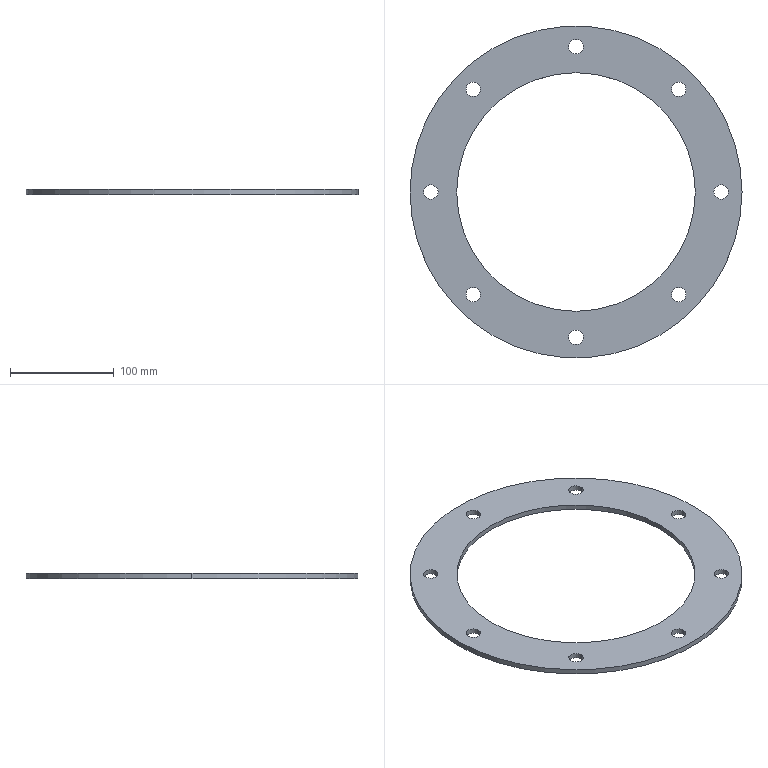Part | SolidWorks | features CirPattern 1, FlatPattern 1, HoleWzd 1, SMBaseFlange 1, SheetMetal 1 | 1 solid | 22 faces | box 320 x 320 x 5 mm | volume 188229 mm3 | cylinder 20 | plane 2 | commonest cylinder face diameters 14 x16 230 x2 320 x2
STEP:
#1=CARTESIAN_POINT('',(91.995,98.995,-5.));
#2=VERTEX_POINT('',#1);
#3=CARTESIAN_POINT('',(105.995,98.995,-5.));
#4=VERTEX_POINT('',#3);
#5=CARTESIAN_POINT('',(98.995,98.995,-5.));
#6=DIRECTION('',(0.,0.,1.));
#7=DIRECTION('',(1.,0.,0.));
#8=AXIS2_PLACEMENT_3D('',#5,#6,#7);
#9=CIRCLE('',#8,7.);
#10=EDGE_CURVE('',#2,#4,#9,.T.);
#11=ORIENTED_EDGE('',*,*,#10,.F.);
#12=CARTESIAN_POINT('',(91.995,98.995,0.));
#13=VERTEX_POINT('',#12);
#14=CARTESIAN_POINT('',(91.995,98.995,0.));
#15=DIRECTION('',(0.,0.,1.));
#16=VECTOR('',#15,1000.);
#17=LINE('',#14,#16);
#18=EDGE_CURVE('',#2,#13,#17,.T.);
#19=ORIENTED_EDGE('',*,*,#18,.T.);
#20=CARTESIAN_POINT('',(105.995,98.995,0.));
#21=VERTEX_POINT('',#20);
#22=CARTESIAN_POINT('',(98.995,98.995,0.));
#23=DIRECTION('',(0.,0.,1.));
#24=DIRECTION('',(1.,0.,0.));
#25=AXIS2_PLACEMENT_3D('',#22,#23,#24);
#26=CIRCLE('',#25,7.);
#27=EDGE_CURVE('',#13,#21,#26,.T.);
#28=ORIENTED_EDGE('',*,*,#27,.T.);
#29=CARTESIAN_POINT('',(105.995,98.995,0.));
#30=DIRECTION('',(0.,0.,1.));
#31=VECTOR('',#30,1000.);
#32=LINE('',#29,#31);
#33=EDGE_CURVE('',#4,#21,#32,.T.);
#34=ORIENTED_EDGE('',*,*,#33,.F.);
#35=EDGE_LOOP('',(#11,#19,#28,#34));
#36=FACE_OUTER_BOUND('',#35,.T.);
#37=CARTESIAN_POINT('',(98.995,98.995,0.));
#38=DIRECTION('',(0.,0.,1.));
#39=DIRECTION('',(1.,0.,0.));
#40=AXIS2_PLACEMENT_3D('',#37,#38,#39);
#41=CYLINDRICAL_SURFACE('',#40,7.);
#42=ADVANCED_FACE('',(#36),#41,.F.);
#43=CARTESIAN_POINT('',(133.,0.,-5.));
#44=VERTEX_POINT('',#43);
#45=CARTESIAN_POINT('',(147.,0.,-5.));
#46=VERTEX_POINT('',#45);
#47=CARTESIAN_POINT('',(140.,0.,-5.));
#48=DIRECTION('',(0.,0.,1.));
#49=DIRECTION('',(1.,0.,0.));
#50=AXIS2_PLACEMENT_3D('',#47,#48,#49);
#51=CIRCLE('',#50,7.);
#52=EDGE_CURVE('',#44,#46,#51,.T.);
#53=ORIENTED_EDGE('',*,*,#52,.F.);
#54=CARTESIAN_POINT('',(133.,0.,0.));
#55=VERTEX_POINT('',#54);
#56=CARTESIAN_POINT('',(133.,0.,0.));
#57=DIRECTION('',(0.,0.,1.));
#58=VECTOR('',#57,1000.);
#59=LINE('',#56,#58);
#60=EDGE_CURVE('',#44,#55,#59,.T.);
#61=ORIENTED_EDGE('',*,*,#60,.T.);
#62=CARTESIAN_POINT('',(147.,0.,0.));
#63=VERTEX_POINT('',#62);
#64=CARTESIAN_POINT('',(140.,0.,0.));
#65=DIRECTION('',(0.,0.,1.));
#66=DIRECTION('',(1.,0.,0.));
#67=AXIS2_PLACEMENT_3D('',#64,#65,#66);
#68=CIRCLE('',#67,7.);
#69=EDGE_CURVE('',#55,#63,#68,.T.);
#70=ORIENTED_EDGE('',*,*,#69,.T.);
#71=CARTESIAN_POINT('',(147.,0.,0.));
#72=DIRECTION('',(0.,0.,1.));
#73=VECTOR('',#72,1000.);
#74=LINE('',#71,#73);
#75=EDGE_CURVE('',#46,#63,#74,.T.);
#76=ORIENTED_EDGE('',*,*,#75,.F.);
#77=EDGE_LOOP('',(#53,#61,#70,#76));
#78=FACE_OUTER_BOUND('',#77,.T.);
#79=CARTESIAN_POINT('',(140.,0.,0.));
#80=DIRECTION('',(0.,0.,1.));
#81=DIRECTION('',(1.,0.,0.));
#82=AXIS2_PLACEMENT_3D('',#79,#80,#81);
#83=CYLINDRICAL_SURFACE('',#82,7.);
#84=ADVANCED_FACE('',(#78),#83,.F.);
#85=CARTESIAN_POINT('',(91.995,-98.995,-5.));
#86=VERTEX_POINT('',#85);
#87=CARTESIAN_POINT('',(105.995,-98.995,-5.));
#88=VERTEX_POINT('',#87);
#89=CARTESIAN_POINT('',(98.995,-98.995,-5.));
#90=DIRECTION('',(0.,0.,1.));
#91=DIRECTION('',(1.,0.,0.));
#92=AXIS2_PLACEMENT_3D('',#89,#90,#91);
#93=CIRCLE('',#92,7.);
#94=EDGE_CURVE('',#86,#88,#93,.T.);
#95=ORIENTED_EDGE('',*,*,#94,.F.);
#96=CARTESIAN_POINT('',(91.995,-98.995,0.));
#97=VERTEX_POINT('',#96);
#98=CARTESIAN_POINT('',(91.995,-98.995,0.));
#99=DIRECTION('',(0.,0.,1.));
#100=VECTOR('',#99,1000.);
#101=LINE('',#98,#100);
#102=EDGE_CURVE('',#86,#97,#101,.T.);
#103=ORIENTED_EDGE('',*,*,#102,.T.);
#104=CARTESIAN_POINT('',(105.995,-98.995,0.));
#105=VERTEX_POINT('',#104);
#106=CARTESIAN_POINT('',(98.995,-98.995,0.));
#107=DIRECTION('',(0.,0.,1.));
#108=DIRECTION('',(1.,0.,0.));
#109=AXIS2_PLACEMENT_3D('',#106,#107,#108);
#110=CIRCLE('',#109,7.);
#111=EDGE_CURVE('',#97,#105,#110,.T.);
#112=ORIENTED_EDGE('',*,*,#111,.T.);
#113=CARTESIAN_POINT('',(105.995,-98.995,0.));
#114=DIRECTION('',(0.,0.,1.));
#115=VECTOR('',#114,1000.);
#116=LINE('',#113,#115);
#117=EDGE_CURVE('',#88,#105,#116,.T.);
#118=ORIENTED_EDGE('',*,*,#117,.F.);
#119=EDGE_LOOP('',(#95,#103,#112,#118));
#120=FACE_OUTER_BOUND('',#119,.T.);
#121=CARTESIAN_POINT('',(98.995,-98.995,0.));
#122=DIRECTION('',(0.,0.,1.));
#123=DIRECTION('',(1.,0.,0.));
#124=AXIS2_PLACEMENT_3D('',#121,#122,#123);
#125=CYLINDRICAL_SURFACE('',#124,7.);
#126=ADVANCED_FACE('',(#120),#125,.F.);
#127=CARTESIAN_POINT('',(-7.,-140.,-5.));
#128=VERTEX_POINT('',#127);
#129=CARTESIAN_POINT('',(7.,-140.,-5.));
#130=VERTEX_POINT('',#129);
#131=CARTESIAN_POINT('',(0.,-140.,-5.));
#132=DIRECTION('',(0.,0.,1.));
#133=DIRECTION('',(1.,0.,0.));
#134=AXIS2_PLACEMENT_3D('',#131,#132,#133);
#135=CIRCLE('',#134,7.);
#136=EDGE_CURVE('',#128,#130,#135,.T.);
#137=ORIENTED_EDGE('',*,*,#136,.F.);
#138=CARTESIAN_POINT('',(-7.,-140.,0.));
#139=VERTEX_POINT('',#138);
#140=CARTESIAN_POINT('',(-7.,-140.,0.));
#141=DIRECTION('',(0.,0.,1.));
#142=VECTOR('',#141,1000.);
#143=LINE('',#140,#142);
#144=EDGE_CURVE('',#128,#139,#143,.T.);
#145=ORIENTED_EDGE('',*,*,#144,.T.);
#146=CARTESIAN_POINT('',(7.,-140.,0.));
#147=VERTEX_POINT('',#146);
#148=CARTESIAN_POINT('',(0.,-140.,0.));
#149=DIRECTION('',(0.,0.,1.));
#150=DIRECTION('',(1.,0.,0.));
#151=AXIS2_PLACEMENT_3D('',#148,#149,#150);
#152=CIRCLE('',#151,7.);
#153=EDGE_CURVE('',#139,#147,#152,.T.);
#154=ORIENTED_EDGE('',*,*,#153,.T.);
#155=CARTESIAN_POINT('',(7.,-140.,0.));
#156=DIRECTION('',(0.,0.,1.));
#157=VECTOR('',#156,1000.);
#158=LINE('',#155,#157);
#159=EDGE_CURVE('',#130,#147,#158,.T.);
#160=ORIENTED_EDGE('',*,*,#159,.F.);
#161=EDGE_LOOP('',(#137,#145,#154,#160));
#162=FACE_OUTER_BOUND('',#161,.T.);
#163=CARTESIAN_POINT('',(0.,-140.,0.));
#164=DIRECTION('',(0.,0.,1.));
#165=DIRECTION('',(1.,0.,0.));
#166=AXIS2_PLACEMENT_3D('',#163,#164,#165);
#167=CYLINDRICAL_SURFACE('',#166,7.);
#168=ADVANCED_FACE('',(#162),#167,.F.);
#169=CARTESIAN_POINT('',(-105.995,-98.995,-5.));
#170=VERTEX_POINT('',#169);
#171=CARTESIAN_POINT('',(-91.995,-98.995,-5.));
#172=VERTEX_POINT('',#171);
#173=CARTESIAN_POINT('',(-98.995,-98.995,-5.));
#174=DIRECTION('',(0.,0.,1.));
#175=DIRECTION('',(1.,0.,0.));
#176=AXIS2_PLACEMENT_3D('',#173,#174,#175);
#177=CIRCLE('',#176,7.);
#178=EDGE_CURVE('',#170,#172,#177,.T.);
#179=ORIENTED_EDGE('',*,*,#178,.F.);
#180=CARTESIAN_POINT('',(-105.995,-98.995,0.));
#181=VERTEX_POINT('',#180);
#182=CARTESIAN_POINT('',(-105.995,-98.995,0.));
#183=DIRECTION('',(0.,0.,1.));
#184=VECTOR('',#183,1000.);
#185=LINE('',#182,#184);
#186=EDGE_CURVE('',#170,#181,#185,.T.);
#187=ORIENTED_EDGE('',*,*,#186,.T.);
#188=CARTESIAN_POINT('',(-91.995,-98.995,0.));
#189=VERTEX_POINT('',#188);
#190=CARTESIAN_POINT('',(-98.995,-98.995,0.));
#191=DIRECTION('',(0.,0.,1.));
#192=DIRECTION('',(1.,0.,0.));
#193=AXIS2_PLACEMENT_3D('',#190,#191,#192);
#194=CIRCLE('',#193,7.);
#195=EDGE_CURVE('',#181,#189,#194,.T.);
#196=ORIENTED_EDGE('',*,*,#195,.T.);
#197=CARTESIAN_POINT('',(-91.995,-98.995,0.));
#198=DIRECTION('',(0.,0.,1.));
#199=VECTOR('',#198,1000.);
#200=LINE('',#197,#199);
#201=EDGE_CURVE('',#172,#189,#200,.T.);
#202=ORIENTED_EDGE('',*,*,#201,.F.);
#203=EDGE_LOOP('',(#179,#187,#196,#202));
#204=FACE_OUTER_BOUND('',#203,.T.);
#205=CARTESIAN_POINT('',(-98.995,-98.995,0.));
#206=DIRECTION('',(0.,0.,1.));
#207=DIRECTION('',(1.,0.,0.));
#208=AXIS2_PLACEMENT_3D('',#205,#206,#207);
#209=CYLINDRICAL_SURFACE('',#208,7.);
#210=ADVANCED_FACE('',(#204),#209,.F.);
#211=CARTESIAN_POINT('',(-147.,0.,-5.));
#212=VERTEX_POINT('',#211);
#213=CARTESIAN_POINT('',(-133.,0.,-5.));
#214=VERTEX_POINT('',#213);
#215=CARTESIAN_POINT('',(-140.,0.,-5.));
#216=DIRECTION('',(0.,0.,1.));
#217=DIRECTION('',(1.,0.,0.));
#218=AXIS2_PLACEMENT_3D('',#215,#216,#217);
#219=CIRCLE('',#218,7.);
#220=EDGE_CURVE('',#212,#214,#219,.T.);
#221=ORIENTED_EDGE('',*,*,#220,.F.);
#222=CARTESIAN_POINT('',(-147.,0.,0.));
#223=VERTEX_POINT('',#222);
#224=CARTESIAN_POINT('',(-147.,0.,0.));
#225=DIRECTION('',(0.,0.,1.));
#226=VECTOR('',#225,1000.);
#227=LINE('',#224,#226);
#228=EDGE_CURVE('',#212,#223,#227,.T.);
#229=ORIENTED_EDGE('',*,*,#228,.T.);
#230=CARTESIAN_POINT('',(-133.,0.,0.));
#231=VERTEX_POINT('',#230);
#232=CARTESIAN_POINT('',(-140.,0.,0.));
#233=DIRECTION('',(0.,0.,1.));
#234=DIRECTION('',(1.,0.,0.));
#235=AXIS2_PLACEMENT_3D('',#232,#233,#234);
#236=CIRCLE('',#235,7.);
#237=EDGE_CURVE('',#223,#231,#236,.T.);
#238=ORIENTED_EDGE('',*,*,#237,.T.);
#239=CARTESIAN_POINT('',(-133.,0.,0.));
#240=DIRECTION('',(0.,0.,1.));
#241=VECTOR('',#240,1000.);
#242=LINE('',#239,#241);
#243=EDGE_CURVE('',#214,#231,#242,.T.);
#244=ORIENTED_EDGE('',*,*,#243,.F.);
#245=EDGE_LOOP('',(#221,#229,#238,#244));
#246=FACE_OUTER_BOUND('',#245,.T.);
#247=CARTESIAN_POINT('',(-140.,0.,0.));
#248=DIRECTION('',(0.,0.,1.));
#249=DIRECTION('',(1.,0.,0.));
#250=AXIS2_PLACEMENT_3D('',#247,#248,#249);
#251=CYLINDRICAL_SURFACE('',#250,7.);
#252=ADVANCED_FACE('',(#246),#251,.F.);
#253=CARTESIAN_POINT('',(-105.995,98.995,-5.));
#254=VERTEX_POINT('',#253);
#255=CARTESIAN_POINT('',(-91.995,98.995,-5.));
#256=VERTEX_POINT('',#255);
#257=CARTESIAN_POINT('',(-98.995,98.995,-5.));
#258=DIRECTION('',(0.,0.,1.));
#259=DIRECTION('',(1.,0.,0.));
#260=AXIS2_PLACEMENT_3D('',#257,#258,#259);
#261=CIRCLE('',#260,7.);
#262=EDGE_CURVE('',#254,#256,#261,.T.);
#263=ORIENTED_EDGE('',*,*,#262,.F.);
#264=CARTESIAN_POINT('',(-105.995,98.995,0.));
#265=VERTEX_POINT('',#264);
#266=CARTESIAN_POINT('',(-105.995,98.995,0.));
#267=DIRECTION('',(0.,0.,1.));
#268=VECTOR('',#267,1000.);
#269=LINE('',#266,#268);
#270=EDGE_CURVE('',#254,#265,#269,.T.);
#271=ORIENTED_EDGE('',*,*,#270,.T.);
#272=CARTESIAN_POINT('',(-91.995,98.995,0.));
#273=VERTEX_POINT('',#272);
#274=CARTESIAN_POINT('',(-98.995,98.995,0.));
#275=DIRECTION('',(0.,0.,1.));
#276=DIRECTION('',(1.,0.,0.));
#277=AXIS2_PLACEMENT_3D('',#274,#275,#276);
#278=CIRCLE('',#277,7.);
#279=EDGE_CURVE('',#265,#273,#278,.T.);
#280=ORIENTED_EDGE('',*,*,#279,.T.);
#281=CARTESIAN_POINT('',(-91.995,98.995,0.));
#282=DIRECTION('',(0.,0.,1.));
#283=VECTOR('',#282,1000.);
#284=LINE('',#281,#283);
#285=EDGE_CURVE('',#256,#273,#284,.T.);
#286=ORIENTED_EDGE('',*,*,#285,.F.);
#287=EDGE_LOOP('',(#263,#271,#280,#286));
#288=FACE_OUTER_BOUND('',#287,.T.);
#289=CARTESIAN_POINT('',(-98.995,98.995,0.));
#290=DIRECTION('',(0.,0.,1.));
#291=DIRECTION('',(1.,0.,0.));
#292=AXIS2_PLACEMENT_3D('',#289,#290,#291);
#293=CYLINDRICAL_SURFACE('',#292,7.);
#294=ADVANCED_FACE('',(#288),#293,.F.);
#295=CARTESIAN_POINT('',(-7.,140.,-5.));
#296=VERTEX_POINT('',#295);
#297=CARTESIAN_POINT('',(7.,140.,-5.));
#298=VERTEX_POINT('',#297);
#299=CARTESIAN_POINT('',(0.,140.,-5.));
#300=DIRECTION('',(0.,0.,1.));
#301=DIRECTION('',(1.,0.,0.));
#302=AXIS2_PLACEMENT_3D('',#299,#300,#301);
#303=CIRCLE('',#302,7.);
#304=EDGE_CURVE('',#296,#298,#303,.T.);
#305=ORIENTED_EDGE('',*,*,#304,.F.);
#306=CARTESIAN_POINT('',(-7.,140.,0.));
#307=VERTEX_POINT('',#306);
#308=CARTESIAN_POINT('',(-7.,140.,0.));
#309=DIRECTION('',(0.,0.,1.));
#310=VECTOR('',#309,1000.);
#311=LINE('',#308,#310);
#312=EDGE_CURVE('',#296,#307,#311,.T.);
#313=ORIENTED_EDGE('',*,*,#312,.T.);
#314=CARTESIAN_POINT('',(7.,140.,0.));
#315=VERTEX_POINT('',#314);
#316=CARTESIAN_POINT('',(0.,140.,0.));
#317=DIRECTION('',(0.,0.,1.));
#318=DIRECTION('',(1.,0.,0.));
#319=AXIS2_PLACEMENT_3D('',#316,#317,#318);
#320=CIRCLE('',#319,7.);
#321=EDGE_CURVE('',#307,#315,#320,.T.);
#322=ORIENTED_EDGE('',*,*,#321,.T.);
#323=CARTESIAN_POINT('',(7.,140.,0.));
#324=DIRECTION('',(0.,0.,1.));
#325=VECTOR('',#324,1000.);
#326=LINE('',#323,#325);
#327=EDGE_CURVE('',#298,#315,#326,.T.);
#328=ORIENTED_EDGE('',*,*,#327,.F.);
#329=EDGE_LOOP('',(#305,#313,#322,#328));
#330=FACE_OUTER_BOUND('',#329,.T.);
#331=CARTESIAN_POINT('',(0.,140.,0.));
#332=DIRECTION('',(0.,0.,1.));
#333=DIRECTION('',(1.,0.,0.));
#334=AXIS2_PLACEMENT_3D('',#331,#332,#333);
#335=CYLINDRICAL_SURFACE('',#334,7.);
#336=ADVANCED_FACE('',(#330),#335,.F.);
#337=CARTESIAN_POINT('',(-115.,0.,-5.));
#338=VERTEX_POINT('',#337);
#339=CARTESIAN_POINT('',(115.,0.,-5.));
#340=VERTEX_POINT('',#339);
#341=CARTESIAN_POINT('',(0.,0.,-5.));
#342=DIRECTION('',(0.,0.,1.));
#343=DIRECTION('',(1.,0.,0.));
#344=AXIS2_PLACEMENT_3D('',#341,#342,#343);
#345=CIRCLE('',#344,115.);
#346=EDGE_CURVE('',#338,#340,#345,.T.);
#347=ORIENTED_EDGE('',*,*,#346,.F.);
#348=CARTESIAN_POINT('',(-115.,0.,0.));
#349=VERTEX_POINT('',#348);
#350=CARTESIAN_POINT('',(-115.,0.,-5.));
#351=DIRECTION('',(0.,0.,1.));
#352=VECTOR('',#351,1000.);
#353=LINE('',#350,#352);
#354=EDGE_CURVE('',#338,#349,#353,.T.);
#355=ORIENTED_EDGE('',*,*,#354,.T.);
#356=CARTESIAN_POINT('',(115.,0.,0.));
#357=VERTEX_POINT('',#356);
#358=CARTESIAN_POINT('',(0.,0.,0.));
#359=DIRECTION('',(0.,0.,1.));
#360=DIRECTION('',(1.,0.,0.));
#361=AXIS2_PLACEMENT_3D('',#358,#359,#360);
#362=CIRCLE('',#361,115.);
#363=EDGE_CURVE('',#349,#357,#362,.T.);
#364=ORIENTED_EDGE('',*,*,#363,.T.);
#365=CARTESIAN_POINT('',(115.,0.,-5.));
#366=DIRECTION('',(0.,0.,1.));
#367=VECTOR('',#366,1000.);
#368=LINE('',#365,#367);
#369=EDGE_CURVE('',#340,#357,#368,.T.);
#370=ORIENTED_EDGE('',*,*,#369,.F.);
#371=EDGE_LOOP('',(#347,#355,#364,#370));
#372=FACE_OUTER_BOUND('',#371,.T.);
#373=CARTESIAN_POINT('',(0.,0.,-5.));
#374=DIRECTION('',(0.,0.,1.));
#375=DIRECTION('',(1.,0.,0.));
#376=AXIS2_PLACEMENT_3D('',#373,#374,#375);
#377=CYLINDRICAL_SURFACE('',#376,115.);
#378=ADVANCED_FACE('',(#372),#377,.F.);
#379=CARTESIAN_POINT('',(160.,0.,-5.));
#380=VERTEX_POINT('',#379);
#381=CARTESIAN_POINT('',(-160.,0.,-5.));
#382=VERTEX_POINT('',#381);
#383=CARTESIAN_POINT('',(0.,0.,-5.));
#384=DIRECTION('',(0.,0.,1.));
#385=DIRECTION('',(1.,0.,0.));
#386=AXIS2_PLACEMENT_3D('',#383,#384,#385);
#387=CIRCLE('',#386,160.);
#388=EDGE_CURVE('',#380,#382,#387,.T.);
#389=ORIENTED_EDGE('',*,*,#388,.T.);
#390=CARTESIAN_POINT('',(-160.,0.,0.));
#391=VERTEX_POINT('',#390);
#392=CARTESIAN_POINT('',(-160.,0.,-5.));
#393=DIRECTION('',(0.,0.,1.));
#394=VECTOR('',#393,1000.);
#395=LINE('',#392,#394);
#396=EDGE_CURVE('',#382,#391,#395,.T.);
#397=ORIENTED_EDGE('',*,*,#396,.T.);
#398=CARTESIAN_POINT('',(160.,0.,0.));
#399=VERTEX_POINT('',#398);
#400=CARTESIAN_POINT('',(0.,0.,0.));
#401=DIRECTION('',(0.,0.,1.));
#402=DIRECTION('',(1.,0.,0.));
#403=AXIS2_PLACEMENT_3D('',#400,#401,#402);
#404=CIRCLE('',#403,160.);
#405=EDGE_CURVE('',#399,#391,#404,.T.);
#406=ORIENTED_EDGE('',*,*,#405,.F.);
#407=CARTESIAN_POINT('',(160.,0.,-5.));
#408=DIRECTION('',(0.,0.,1.));
#409=VECTOR('',#408,1000.);
#410=LINE('',#407,#409);
#411=EDGE_CURVE('',#380,#399,#410,.T.);
#412=ORIENTED_EDGE('',*,*,#411,.F.);
#413=EDGE_LOOP('',(#389,#397,#406,#412));
#414=FACE_OUTER_BOUND('',#413,.T.);
#415=CARTESIAN_POINT('',(0.,0.,-5.));
#416=DIRECTION('',(0.,0.,1.));
#417=DIRECTION('',(1.,0.,0.));
#418=AXIS2_PLACEMENT_3D('',#415,#416,#417);
#419=CYLINDRICAL_SURFACE('',#418,160.);
#420=ADVANCED_FACE('',(#414),#419,.T.);
#421=ORIENTED_EDGE('',*,*,#396,.F.);
#422=CARTESIAN_POINT('',(0.,0.,-5.));
#423=DIRECTION('',(0.,0.,1.));
#424=DIRECTION('',(1.,0.,0.));
#425=AXIS2_PLACEMENT_3D('',#422,#423,#424);
#426=CIRCLE('',#425,160.);
#427=EDGE_CURVE('',#382,#380,#426,.T.);
#428=ORIENTED_EDGE('',*,*,#427,.T.);
#429=ORIENTED_EDGE('',*,*,#411,.T.);
#430=CARTESIAN_POINT('',(0.,0.,0.));
#431=DIRECTION('',(0.,0.,1.));
#432=DIRECTION('',(1.,0.,0.));
#433=AXIS2_PLACEMENT_3D('',#430,#431,#432);
#434=CIRCLE('',#433,160.);
#435=EDGE_CURVE('',#391,#399,#434,.T.);
#436=ORIENTED_EDGE('',*,*,#435,.F.);
#437=EDGE_LOOP('',(#421,#428,#429,#436));
#438=FACE_OUTER_BOUND('',#437,.T.);
#439=CARTESIAN_POINT('',(0.,0.,-5.));
#440=DIRECTION('',(0.,0.,1.));
#441=DIRECTION('',(1.,0.,0.));
#442=AXIS2_PLACEMENT_3D('',#439,#440,#441);
#443=CYLINDRICAL_SURFACE('',#442,160.);
#444=ADVANCED_FACE('',(#438),#443,.T.);
#445=CARTESIAN_POINT('',(98.995,98.995,-5.));
#446=DIRECTION('',(0.,0.,1.));
#447=DIRECTION('',(1.,0.,0.));
#448=AXIS2_PLACEMENT_3D('',#445,#446,#447);
#449=CIRCLE('',#448,7.);
#450=EDGE_CURVE('',#4,#2,#449,.T.);
#451=ORIENTED_EDGE('',*,*,#450,.T.);
#452=ORIENTED_EDGE('',*,*,#10,.T.);
#453=EDGE_LOOP('',(#451,#452));
#454=FACE_BOUND('',#453,.T.);
#455=CARTESIAN_POINT('',(140.,0.,-5.));
#456=DIRECTION('',(0.,0.,1.));
#457=DIRECTION('',(1.,0.,0.));
#458=AXIS2_PLACEMENT_3D('',#455,#456,#457);
#459=CIRCLE('',#458,7.);
#460=EDGE_CURVE('',#46,#44,#459,.T.);
#461=ORIENTED_EDGE('',*,*,#460,.T.);
#462=ORIENTED_EDGE('',*,*,#52,.T.);
#463=EDGE_LOOP('',(#461,#462));
#464=FACE_BOUND('',#463,.T.);
#465=CARTESIAN_POINT('',(98.995,-98.995,-5.));
#466=DIRECTION('',(0.,0.,1.));
#467=DIRECTION('',(1.,0.,0.));
#468=AXIS2_PLACEMENT_3D('',#465,#466,#467);
#469=CIRCLE('',#468,7.);
#470=EDGE_CURVE('',#88,#86,#469,.T.);
#471=ORIENTED_EDGE('',*,*,#470,.T.);
#472=ORIENTED_EDGE('',*,*,#94,.T.);
#473=EDGE_LOOP('',(#471,#472));
#474=FACE_BOUND('',#473,.T.);
#475=CARTESIAN_POINT('',(0.,-140.,-5.));
#476=DIRECTION('',(0.,0.,1.));
#477=DIRECTION('',(1.,0.,0.));
#478=AXIS2_PLACEMENT_3D('',#475,#476,#477);
#479=CIRCLE('',#478,7.);
#480=EDGE_CURVE('',#130,#128,#479,.T.);
#481=ORIENTED_EDGE('',*,*,#480,.T.);
#482=ORIENTED_EDGE('',*,*,#136,.T.);
#483=EDGE_LOOP('',(#481,#482));
#484=FACE_BOUND('',#483,.T.);
#485=CARTESIAN_POINT('',(-98.995,-98.995,-5.));
#486=DIRECTION('',(0.,0.,1.));
#487=DIRECTION('',(1.,0.,0.));
#488=AXIS2_PLACEMENT_3D('',#485,#486,#487);
#489=CIRCLE('',#488,7.);
#490=EDGE_CURVE('',#172,#170,#489,.T.);
#491=ORIENTED_EDGE('',*,*,#490,.T.);
#492=ORIENTED_EDGE('',*,*,#178,.T.);
#493=EDGE_LOOP('',(#491,#492));
#494=FACE_BOUND('',#493,.T.);
#495=CARTESIAN_POINT('',(-140.,0.,-5.));
#496=DIRECTION('',(0.,0.,1.));
#497=DIRECTION('',(1.,0.,0.));
#498=AXIS2_PLACEMENT_3D('',#495,#496,#497);
#499=CIRCLE('',#498,7.);
#500=EDGE_CURVE('',#214,#212,#499,.T.);
#501=ORIENTED_EDGE('',*,*,#500,.T.);
#502=ORIENTED_EDGE('',*,*,#220,.T.);
#503=EDGE_LOOP('',(#501,#502));
#504=FACE_BOUND('',#503,.T.);
#505=CARTESIAN_POINT('',(-98.995,98.995,-5.));
#506=DIRECTION('',(0.,0.,1.));
#507=DIRECTION('',(1.,0.,0.));
#508=AXIS2_PLACEMENT_3D('',#505,#506,#507);
#509=CIRCLE('',#508,7.);
#510=EDGE_CURVE('',#256,#254,#509,.T.);
#511=ORIENTED_EDGE('',*,*,#510,.T.);
#512=ORIENTED_EDGE('',*,*,#262,.T.);
#513=EDGE_LOOP('',(#511,#512));
#514=FACE_BOUND('',#513,.T.);
#515=CARTESIAN_POINT('',(0.,140.,-5.));
#516=DIRECTION('',(0.,0.,1.));
#517=DIRECTION('',(1.,0.,0.));
#518=AXIS2_PLACEMENT_3D('',#515,#516,#517);
#519=CIRCLE('',#518,7.);
#520=EDGE_CURVE('',#298,#296,#519,.T.);
#521=ORIENTED_EDGE('',*,*,#520,.T.);
#522=ORIENTED_EDGE('',*,*,#304,.T.);
#523=EDGE_LOOP('',(#521,#522));
#524=FACE_BOUND('',#523,.T.);
#525=CARTESIAN_POINT('',(0.,0.,-5.));
#526=DIRECTION('',(0.,0.,1.));
#527=DIRECTION('',(1.,0.,0.));
#528=AXIS2_PLACEMENT_3D('',#525,#526,#527);
#529=CIRCLE('',#528,115.);
#530=EDGE_CURVE('',#340,#338,#529,.T.);
#531=ORIENTED_EDGE('',*,*,#530,.T.);
#532=ORIENTED_EDGE('',*,*,#346,.T.);
#533=EDGE_LOOP('',(#531,#532));
#534=FACE_BOUND('',#533,.T.);
#535=ORIENTED_EDGE('',*,*,#388,.F.);
#536=ORIENTED_EDGE('',*,*,#427,.F.);
#537=EDGE_LOOP('',(#535,#536));
#538=FACE_OUTER_BOUND('',#537,.T.);
#539=CARTESIAN_POINT('',(0.,0.,-5.));
#540=DIRECTION('',(0.,0.,1.));
#541=DIRECTION('',(1.,0.,0.));
#542=AXIS2_PLACEMENT_3D('',#539,#540,#541);
#543=PLANE('',#542);
#544=ADVANCED_FACE('',(#454,#464,#474,#484,#494,#504,#514,#524,#534,#538),#543,.F.);
#545=CARTESIAN_POINT('',(98.995,98.995,0.));
#546=DIRECTION('',(0.,0.,1.));
#547=DIRECTION('',(1.,0.,0.));
#548=AXIS2_PLACEMENT_3D('',#545,#546,#547);
#549=CIRCLE('',#548,7.);
#550=EDGE_CURVE('',#21,#13,#549,.T.);
#551=ORIENTED_EDGE('',*,*,#550,.F.);
#552=ORIENTED_EDGE('',*,*,#27,.F.);
#553=EDGE_LOOP('',(#551,#552));
#554=FACE_BOUND('',#553,.T.);
#555=CARTESIAN_POINT('',(140.,0.,0.));
#556=DIRECTION('',(0.,0.,1.));
#557=DIRECTION('',(1.,0.,0.));
#558=AXIS2_PLACEMENT_3D('',#555,#556,#557);
#559=CIRCLE('',#558,7.);
#560=EDGE_CURVE('',#63,#55,#559,.T.);
#561=ORIENTED_EDGE('',*,*,#560,.F.);
#562=ORIENTED_EDGE('',*,*,#69,.F.);
#563=EDGE_LOOP('',(#561,#562));
#564=FACE_BOUND('',#563,.T.);
#565=CARTESIAN_POINT('',(98.995,-98.995,0.));
#566=DIRECTION('',(0.,0.,1.));
#567=DIRECTION('',(1.,0.,0.));
#568=AXIS2_PLACEMENT_3D('',#565,#566,#567);
#569=CIRCLE('',#568,7.);
#570=EDGE_CURVE('',#105,#97,#569,.T.);
#571=ORIENTED_EDGE('',*,*,#570,.F.);
#572=ORIENTED_EDGE('',*,*,#111,.F.);
#573=EDGE_LOOP('',(#571,#572));
#574=FACE_BOUND('',#573,.T.);
#575=CARTESIAN_POINT('',(0.,-140.,0.));
#576=DIRECTION('',(0.,0.,1.));
#577=DIRECTION('',(1.,0.,0.));
#578=AXIS2_PLACEMENT_3D('',#575,#576,#577);
#579=CIRCLE('',#578,7.);
#580=EDGE_CURVE('',#147,#139,#579,.T.);
#581=ORIENTED_EDGE('',*,*,#580,.F.);
#582=ORIENTED_EDGE('',*,*,#153,.F.);
#583=EDGE_LOOP('',(#581,#582));
#584=FACE_BOUND('',#583,.T.);
#585=CARTESIAN_POINT('',(-98.995,-98.995,0.));
#586=DIRECTION('',(0.,0.,1.));
#587=DIRECTION('',(1.,0.,0.));
#588=AXIS2_PLACEMENT_3D('',#585,#586,#587);
#589=CIRCLE('',#588,7.);
#590=EDGE_CURVE('',#189,#181,#589,.T.);
#591=ORIENTED_EDGE('',*,*,#590,.F.);
#592=ORIENTED_EDGE('',*,*,#195,.F.);
#593=EDGE_LOOP('',(#591,#592));
#594=FACE_BOUND('',#593,.T.);
#595=CARTESIAN_POINT('',(-140.,0.,0.));
#596=DIRECTION('',(0.,0.,1.));
#597=DIRECTION('',(1.,0.,0.));
#598=AXIS2_PLACEMENT_3D('',#595,#596,#597);
#599=CIRCLE('',#598,7.);
#600=EDGE_CURVE('',#231,#223,#599,.T.);
#601=ORIENTED_EDGE('',*,*,#600,.F.);
#602=ORIENTED_EDGE('',*,*,#237,.F.);
#603=EDGE_LOOP('',(#601,#602));
#604=FACE_BOUND('',#603,.T.);
#605=CARTESIAN_POINT('',(-98.995,98.995,0.));
#606=DIRECTION('',(0.,0.,1.));
#607=DIRECTION('',(1.,0.,0.));
#608=AXIS2_PLACEMENT_3D('',#605,#606,#607);
#609=CIRCLE('',#608,7.);
#610=EDGE_CURVE('',#273,#265,#609,.T.);
#611=ORIENTED_EDGE('',*,*,#610,.F.);
#612=ORIENTED_EDGE('',*,*,#279,.F.);
#613=EDGE_LOOP('',(#611,#612));
#614=FACE_BOUND('',#613,.T.);
#615=CARTESIAN_POINT('',(0.,140.,0.));
#616=DIRECTION('',(0.,0.,1.));
#617=DIRECTION('',(1.,0.,0.));
#618=AXIS2_PLACEMENT_3D('',#615,#616,#617);
#619=CIRCLE('',#618,7.);
#620=EDGE_CURVE('',#315,#307,#619,.T.);
#621=ORIENTED_EDGE('',*,*,#620,.F.);
#622=ORIENTED_EDGE('',*,*,#321,.F.);
#623=EDGE_LOOP('',(#621,#622));
#624=FACE_BOUND('',#623,.T.);
#625=CARTESIAN_POINT('',(0.,0.,0.));
#626=DIRECTION('',(0.,0.,1.));
#627=DIRECTION('',(1.,0.,0.));
#628=AXIS2_PLACEMENT_3D('',#625,#626,#627);
#629=CIRCLE('',#628,115.);
#630=EDGE_CURVE('',#357,#349,#629,.T.);
#631=ORIENTED_EDGE('',*,*,#630,.F.);
#632=ORIENTED_EDGE('',*,*,#363,.F.);
#633=EDGE_LOOP('',(#631,#632));
#634=FACE_BOUND('',#633,.T.);
#635=ORIENTED_EDGE('',*,*,#405,.T.);
#636=ORIENTED_EDGE('',*,*,#435,.T.);
#637=EDGE_LOOP('',(#635,#636));
#638=FACE_OUTER_BOUND('',#637,.T.);
#639=CARTESIAN_POINT('',(0.,0.,0.));
#640=DIRECTION('',(0.,0.,1.));
#641=DIRECTION('',(1.,0.,0.));
#642=AXIS2_PLACEMENT_3D('',#639,#640,#641);
#643=PLANE('',#642);
#644=ADVANCED_FACE('',(#554,#564,#574,#584,#594,#604,#614,#624,#634,#638),#643,.T.);
#645=ORIENTED_EDGE('',*,*,#354,.F.);
#646=ORIENTED_EDGE('',*,*,#530,.F.);
#647=ORIENTED_EDGE('',*,*,#369,.T.);
#648=ORIENTED_EDGE('',*,*,#630,.T.);
#649=EDGE_LOOP('',(#645,#646,#647,#648));
#650=FACE_OUTER_BOUND('',#649,.T.);
#651=CARTESIAN_POINT('',(0.,0.,-5.));
#652=DIRECTION('',(0.,0.,1.));
#653=DIRECTION('',(1.,0.,0.));
#654=AXIS2_PLACEMENT_3D('',#651,#652,#653);
#655=CYLINDRICAL_SURFACE('',#654,115.);
#656=ADVANCED_FACE('',(#650),#655,.F.);
#657=ORIENTED_EDGE('',*,*,#312,.F.);
#658=ORIENTED_EDGE('',*,*,#520,.F.);
#659=ORIENTED_EDGE('',*,*,#327,.T.);
#660=ORIENTED_EDGE('',*,*,#620,.T.);
#661=EDGE_LOOP('',(#657,#658,#659,#660));
#662=FACE_OUTER_BOUND('',#661,.T.);
#663=CARTESIAN_POINT('',(0.,140.,0.));
#664=DIRECTION('',(0.,0.,1.));
#665=DIRECTION('',(1.,0.,0.));
#666=AXIS2_PLACEMENT_3D('',#663,#664,#665);
#667=CYLINDRICAL_SURFACE('',#666,7.);
#668=ADVANCED_FACE('',(#662),#667,.F.);
#669=ORIENTED_EDGE('',*,*,#270,.F.);
#670=ORIENTED_EDGE('',*,*,#510,.F.);
#671=ORIENTED_EDGE('',*,*,#285,.T.);
#672=ORIENTED_EDGE('',*,*,#610,.T.);
#673=EDGE_LOOP('',(#669,#670,#671,#672));
#674=FACE_OUTER_BOUND('',#673,.T.);
#675=CARTESIAN_POINT('',(-98.995,98.995,0.));
#676=DIRECTION('',(0.,0.,1.));
#677=DIRECTION('',(1.,0.,0.));
#678=AXIS2_PLACEMENT_3D('',#675,#676,#677);
#679=CYLINDRICAL_SURFACE('',#678,7.);
#680=ADVANCED_FACE('',(#674),#679,.F.);
#681=ORIENTED_EDGE('',*,*,#228,.F.);
#682=ORIENTED_EDGE('',*,*,#500,.F.);
#683=ORIENTED_EDGE('',*,*,#243,.T.);
#684=ORIENTED_EDGE('',*,*,#600,.T.);
#685=EDGE_LOOP('',(#681,#682,#683,#684));
#686=FACE_OUTER_BOUND('',#685,.T.);
#687=CARTESIAN_POINT('',(-140.,0.,0.));
#688=DIRECTION('',(0.,0.,1.));
#689=DIRECTION('',(1.,0.,0.));
#690=AXIS2_PLACEMENT_3D('',#687,#688,#689);
#691=CYLINDRICAL_SURFACE('',#690,7.);
#692=ADVANCED_FACE('',(#686),#691,.F.);
#693=ORIENTED_EDGE('',*,*,#186,.F.);
#694=ORIENTED_EDGE('',*,*,#490,.F.);
#695=ORIENTED_EDGE('',*,*,#201,.T.);
#696=ORIENTED_EDGE('',*,*,#590,.T.);
#697=EDGE_LOOP('',(#693,#694,#695,#696));
#698=FACE_OUTER_BOUND('',#697,.T.);
#699=CARTESIAN_POINT('',(-98.995,-98.995,0.));
#700=DIRECTION('',(0.,0.,1.));
#701=DIRECTION('',(1.,0.,0.));
#702=AXIS2_PLACEMENT_3D('',#699,#700,#701);
#703=CYLINDRICAL_SURFACE('',#702,7.);
#704=ADVANCED_FACE('',(#698),#703,.F.);
#705=ORIENTED_EDGE('',*,*,#144,.F.);
#706=ORIENTED_EDGE('',*,*,#480,.F.);
#707=ORIENTED_EDGE('',*,*,#159,.T.);
#708=ORIENTED_EDGE('',*,*,#580,.T.);
#709=EDGE_LOOP('',(#705,#706,#707,#708));
#710=FACE_OUTER_BOUND('',#709,.T.);
#711=CARTESIAN_POINT('',(0.,-140.,0.));
#712=DIRECTION('',(0.,0.,1.));
#713=DIRECTION('',(1.,0.,0.));
#714=AXIS2_PLACEMENT_3D('',#711,#712,#713);
#715=CYLINDRICAL_SURFACE('',#714,7.);
#716=ADVANCED_FACE('',(#710),#715,.F.);
#717=ORIENTED_EDGE('',*,*,#102,.F.);
#718=ORIENTED_EDGE('',*,*,#470,.F.);
#719=ORIENTED_EDGE('',*,*,#117,.T.);
#720=ORIENTED_EDGE('',*,*,#570,.T.);
#721=EDGE_LOOP('',(#717,#718,#719,#720));
#722=FACE_OUTER_BOUND('',#721,.T.);
#723=CARTESIAN_POINT('',(98.995,-98.995,0.));
#724=DIRECTION('',(0.,0.,1.));
#725=DIRECTION('',(1.,0.,0.));
#726=AXIS2_PLACEMENT_3D('',#723,#724,#725);
#727=CYLINDRICAL_SURFACE('',#726,7.);
#728=ADVANCED_FACE('',(#722),#727,.F.);
#729=ORIENTED_EDGE('',*,*,#60,.F.);
#730=ORIENTED_EDGE('',*,*,#460,.F.);
#731=ORIENTED_EDGE('',*,*,#75,.T.);
#732=ORIENTED_EDGE('',*,*,#560,.T.);
#733=EDGE_LOOP('',(#729,#730,#731,#732));
#734=FACE_OUTER_BOUND('',#733,.T.);
#735=CARTESIAN_POINT('',(140.,0.,0.));
#736=DIRECTION('',(0.,0.,1.));
#737=DIRECTION('',(1.,0.,0.));
#738=AXIS2_PLACEMENT_3D('',#735,#736,#737);
#739=CYLINDRICAL_SURFACE('',#738,7.);
#740=ADVANCED_FACE('',(#734),#739,.F.);
#741=ORIENTED_EDGE('',*,*,#18,.F.);
#742=ORIENTED_EDGE('',*,*,#450,.F.);
#743=ORIENTED_EDGE('',*,*,#33,.T.);
#744=ORIENTED_EDGE('',*,*,#550,.T.);
#745=EDGE_LOOP('',(#741,#742,#743,#744));
#746=FACE_OUTER_BOUND('',#745,.T.);
#747=CARTESIAN_POINT('',(98.995,98.995,0.));
#748=DIRECTION('',(0.,0.,1.));
#749=DIRECTION('',(1.,0.,0.));
#750=AXIS2_PLACEMENT_3D('',#747,#748,#749);
#751=CYLINDRICAL_SURFACE('',#750,7.);
#752=ADVANCED_FACE('',(#746),#751,.F.);
#753=CLOSED_SHELL('',(#42,#84,#126,#168,#210,#252,#294,#336,#378,#420,#444,#544,#644,#656,#668,#680,#692,#704,#716,#728,#740,#752));
#754=MANIFOLD_SOLID_BREP('',#753);
#755=CARTESIAN_POINT('',(0.,0.,0.));
#756=DIRECTION('',(0.,0.,1.));
#757=DIRECTION('',(1.,0.,0.));
#758=AXIS2_PLACEMENT_3D('',#755,#756,#757);
#759=(LENGTH_UNIT()NAMED_UNIT(*)SI_UNIT(.MILLI.,.METRE.));
#760=UNCERTAINTY_MEASURE_WITH_UNIT(LENGTH_MEASURE(0.00001),#759,'','');
#761=(NAMED_UNIT(*)PLANE_ANGLE_UNIT()SI_UNIT($,.RADIAN.));
#762=(NAMED_UNIT(*)SI_UNIT($,.STERADIAN.)SOLID_ANGLE_UNIT());
#763=(GEOMETRIC_REPRESENTATION_CONTEXT(3)GLOBAL_UNCERTAINTY_ASSIGNED_CONTEXT((#760))GLOBAL_UNIT_ASSIGNED_CONTEXT((#759,#761,#762))REPRESENTATION_CONTEXT('',''));
#764=ADVANCED_BREP_SHAPE_REPRESENTATION('',(#754,#758),#763);